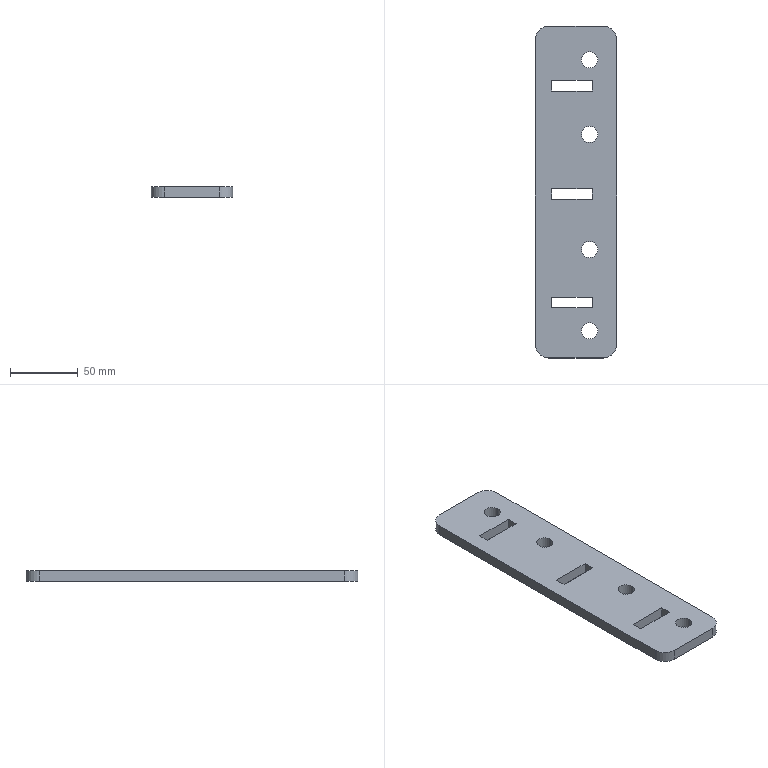Part | SolidWorks | features Fillet 1, FlatPattern 1, SMBaseFlange 1, SheetMetal 1 | 1 solid | 30 faces | box 60 x 245 x 8 mm | volume 107534 mm3 | plane 18 | cylinder 12 | commonest cylinder face diameters 12 x8 20 x4
STEP:
#1=CARTESIAN_POINT('',(88.081,95.,8.));
#2=VERTEX_POINT('',#1);
#3=CARTESIAN_POINT('',(100.081,95.,8.));
#4=VERTEX_POINT('',#3);
#5=CARTESIAN_POINT('',(94.081,95.,8.));
#6=DIRECTION('',(0.,0.,1.));
#7=DIRECTION('',(1.,0.,0.));
#8=AXIS2_PLACEMENT_3D('',#5,#6,#7);
#9=CIRCLE('',#8,6.);
#10=EDGE_CURVE('',#2,#4,#9,.T.);
#11=ORIENTED_EDGE('',*,*,#10,.T.);
#12=CARTESIAN_POINT('',(100.081,95.,0.));
#13=VERTEX_POINT('',#12);
#14=CARTESIAN_POINT('',(100.081,95.,8.));
#15=DIRECTION('',(0.,0.,-1.));
#16=VECTOR('',#15,1000.);
#17=LINE('',#14,#16);
#18=EDGE_CURVE('',#4,#13,#17,.T.);
#19=ORIENTED_EDGE('',*,*,#18,.T.);
#20=CARTESIAN_POINT('',(88.081,95.,0.));
#21=VERTEX_POINT('',#20);
#22=CARTESIAN_POINT('',(94.081,95.,0.));
#23=DIRECTION('',(0.,0.,1.));
#24=DIRECTION('',(1.,0.,0.));
#25=AXIS2_PLACEMENT_3D('',#22,#23,#24);
#26=CIRCLE('',#25,6.);
#27=EDGE_CURVE('',#21,#13,#26,.T.);
#28=ORIENTED_EDGE('',*,*,#27,.F.);
#29=CARTESIAN_POINT('',(88.081,95.,8.));
#30=DIRECTION('',(0.,0.,-1.));
#31=VECTOR('',#30,1000.);
#32=LINE('',#29,#31);
#33=EDGE_CURVE('',#2,#21,#32,.T.);
#34=ORIENTED_EDGE('',*,*,#33,.F.);
#35=EDGE_LOOP('',(#11,#19,#28,#34));
#36=FACE_OUTER_BOUND('',#35,.T.);
#37=CARTESIAN_POINT('',(94.081,95.,8.));
#38=DIRECTION('',(0.,0.,-1.));
#39=DIRECTION('',(-1.,0.,0.));
#40=AXIS2_PLACEMENT_3D('',#37,#38,#39);
#41=CYLINDRICAL_SURFACE('',#40,6.);
#42=ADVANCED_FACE('',(#36),#41,.F.);
#43=CARTESIAN_POINT('',(88.081,40.,8.));
#44=VERTEX_POINT('',#43);
#45=CARTESIAN_POINT('',(100.081,40.,8.));
#46=VERTEX_POINT('',#45);
#47=CARTESIAN_POINT('',(94.081,40.,8.));
#48=DIRECTION('',(0.,0.,1.));
#49=DIRECTION('',(1.,0.,0.));
#50=AXIS2_PLACEMENT_3D('',#47,#48,#49);
#51=CIRCLE('',#50,6.);
#52=EDGE_CURVE('',#44,#46,#51,.T.);
#53=ORIENTED_EDGE('',*,*,#52,.T.);
#54=CARTESIAN_POINT('',(100.081,40.,0.));
#55=VERTEX_POINT('',#54);
#56=CARTESIAN_POINT('',(100.081,40.,8.));
#57=DIRECTION('',(0.,0.,-1.));
#58=VECTOR('',#57,1000.);
#59=LINE('',#56,#58);
#60=EDGE_CURVE('',#46,#55,#59,.T.);
#61=ORIENTED_EDGE('',*,*,#60,.T.);
#62=CARTESIAN_POINT('',(88.081,40.,0.));
#63=VERTEX_POINT('',#62);
#64=CARTESIAN_POINT('',(94.081,40.,0.));
#65=DIRECTION('',(0.,0.,1.));
#66=DIRECTION('',(1.,0.,0.));
#67=AXIS2_PLACEMENT_3D('',#64,#65,#66);
#68=CIRCLE('',#67,6.);
#69=EDGE_CURVE('',#63,#55,#68,.T.);
#70=ORIENTED_EDGE('',*,*,#69,.F.);
#71=CARTESIAN_POINT('',(88.081,40.,8.));
#72=DIRECTION('',(0.,0.,-1.));
#73=VECTOR('',#72,1000.);
#74=LINE('',#71,#73);
#75=EDGE_CURVE('',#44,#63,#74,.T.);
#76=ORIENTED_EDGE('',*,*,#75,.F.);
#77=EDGE_LOOP('',(#53,#61,#70,#76));
#78=FACE_OUTER_BOUND('',#77,.T.);
#79=CARTESIAN_POINT('',(94.081,40.,8.));
#80=DIRECTION('',(0.,0.,-1.));
#81=DIRECTION('',(-1.,0.,0.));
#82=AXIS2_PLACEMENT_3D('',#79,#80,#81);
#83=CYLINDRICAL_SURFACE('',#82,6.);
#84=ADVANCED_FACE('',(#78),#83,.F.);
#85=CARTESIAN_POINT('',(88.081,-45.,8.));
#86=VERTEX_POINT('',#85);
#87=CARTESIAN_POINT('',(100.081,-45.,8.));
#88=VERTEX_POINT('',#87);
#89=CARTESIAN_POINT('',(94.081,-45.,8.));
#90=DIRECTION('',(0.,0.,1.));
#91=DIRECTION('',(1.,0.,0.));
#92=AXIS2_PLACEMENT_3D('',#89,#90,#91);
#93=CIRCLE('',#92,6.);
#94=EDGE_CURVE('',#86,#88,#93,.T.);
#95=ORIENTED_EDGE('',*,*,#94,.T.);
#96=CARTESIAN_POINT('',(100.081,-45.,0.));
#97=VERTEX_POINT('',#96);
#98=CARTESIAN_POINT('',(100.081,-45.,8.));
#99=DIRECTION('',(0.,0.,-1.));
#100=VECTOR('',#99,1000.);
#101=LINE('',#98,#100);
#102=EDGE_CURVE('',#88,#97,#101,.T.);
#103=ORIENTED_EDGE('',*,*,#102,.T.);
#104=CARTESIAN_POINT('',(88.081,-45.,0.));
#105=VERTEX_POINT('',#104);
#106=CARTESIAN_POINT('',(94.081,-45.,0.));
#107=DIRECTION('',(0.,0.,1.));
#108=DIRECTION('',(1.,0.,0.));
#109=AXIS2_PLACEMENT_3D('',#106,#107,#108);
#110=CIRCLE('',#109,6.);
#111=EDGE_CURVE('',#105,#97,#110,.T.);
#112=ORIENTED_EDGE('',*,*,#111,.F.);
#113=CARTESIAN_POINT('',(88.081,-45.,8.));
#114=DIRECTION('',(0.,0.,-1.));
#115=VECTOR('',#114,1000.);
#116=LINE('',#113,#115);
#117=EDGE_CURVE('',#86,#105,#116,.T.);
#118=ORIENTED_EDGE('',*,*,#117,.F.);
#119=EDGE_LOOP('',(#95,#103,#112,#118));
#120=FACE_OUTER_BOUND('',#119,.T.);
#121=CARTESIAN_POINT('',(94.081,-45.,8.));
#122=DIRECTION('',(0.,0.,-1.));
#123=DIRECTION('',(-1.,0.,0.));
#124=AXIS2_PLACEMENT_3D('',#121,#122,#123);
#125=CYLINDRICAL_SURFACE('',#124,6.);
#126=ADVANCED_FACE('',(#120),#125,.F.);
#127=CARTESIAN_POINT('',(88.081,-105.,8.));
#128=VERTEX_POINT('',#127);
#129=CARTESIAN_POINT('',(100.081,-105.,8.));
#130=VERTEX_POINT('',#129);
#131=CARTESIAN_POINT('',(94.081,-105.,8.));
#132=DIRECTION('',(0.,0.,1.));
#133=DIRECTION('',(1.,0.,0.));
#134=AXIS2_PLACEMENT_3D('',#131,#132,#133);
#135=CIRCLE('',#134,6.);
#136=EDGE_CURVE('',#128,#130,#135,.T.);
#137=ORIENTED_EDGE('',*,*,#136,.T.);
#138=CARTESIAN_POINT('',(100.081,-105.,0.));
#139=VERTEX_POINT('',#138);
#140=CARTESIAN_POINT('',(100.081,-105.,8.));
#141=DIRECTION('',(0.,0.,-1.));
#142=VECTOR('',#141,1000.);
#143=LINE('',#140,#142);
#144=EDGE_CURVE('',#130,#139,#143,.T.);
#145=ORIENTED_EDGE('',*,*,#144,.T.);
#146=CARTESIAN_POINT('',(88.081,-105.,0.));
#147=VERTEX_POINT('',#146);
#148=CARTESIAN_POINT('',(94.081,-105.,0.));
#149=DIRECTION('',(0.,0.,1.));
#150=DIRECTION('',(1.,0.,0.));
#151=AXIS2_PLACEMENT_3D('',#148,#149,#150);
#152=CIRCLE('',#151,6.);
#153=EDGE_CURVE('',#147,#139,#152,.T.);
#154=ORIENTED_EDGE('',*,*,#153,.F.);
#155=CARTESIAN_POINT('',(88.081,-105.,8.));
#156=DIRECTION('',(0.,0.,-1.));
#157=VECTOR('',#156,1000.);
#158=LINE('',#155,#157);
#159=EDGE_CURVE('',#128,#147,#158,.T.);
#160=ORIENTED_EDGE('',*,*,#159,.F.);
#161=EDGE_LOOP('',(#137,#145,#154,#160));
#162=FACE_OUTER_BOUND('',#161,.T.);
#163=CARTESIAN_POINT('',(94.081,-105.,8.));
#164=DIRECTION('',(0.,0.,-1.));
#165=DIRECTION('',(-1.,0.,0.));
#166=AXIS2_PLACEMENT_3D('',#163,#164,#165);
#167=CYLINDRICAL_SURFACE('',#166,6.);
#168=ADVANCED_FACE('',(#162),#167,.F.);
#169=ORIENTED_EDGE('',*,*,#52,.F.);
#170=CARTESIAN_POINT('',(94.081,40.,8.));
#171=DIRECTION('',(0.,0.,1.));
#172=DIRECTION('',(1.,0.,0.));
#173=AXIS2_PLACEMENT_3D('',#170,#171,#172);
#174=CIRCLE('',#173,6.);
#175=EDGE_CURVE('',#46,#44,#174,.T.);
#176=ORIENTED_EDGE('',*,*,#175,.F.);
#177=EDGE_LOOP('',(#169,#176));
#178=FACE_BOUND('',#177,.T.);
#179=ORIENTED_EDGE('',*,*,#136,.F.);
#180=CARTESIAN_POINT('',(94.081,-105.,8.));
#181=DIRECTION('',(0.,0.,1.));
#182=DIRECTION('',(1.,0.,0.));
#183=AXIS2_PLACEMENT_3D('',#180,#181,#182);
#184=CIRCLE('',#183,6.);
#185=EDGE_CURVE('',#130,#128,#184,.T.);
#186=ORIENTED_EDGE('',*,*,#185,.F.);
#187=EDGE_LOOP('',(#179,#186));
#188=FACE_BOUND('',#187,.T.);
#189=CARTESIAN_POINT('',(114.081,-115.,8.));
#190=VERTEX_POINT('',#189);
#191=CARTESIAN_POINT('',(114.081,110.,8.));
#192=VERTEX_POINT('',#191);
#193=CARTESIAN_POINT('',(114.081,-125.,8.));
#194=DIRECTION('',(0.,1.,0.));
#195=VECTOR('',#194,1000.);
#196=LINE('',#193,#195);
#197=EDGE_CURVE('',#190,#192,#196,.T.);
#198=ORIENTED_EDGE('',*,*,#197,.T.);
#199=CARTESIAN_POINT('',(104.081,120.,8.));
#200=VERTEX_POINT('',#199);
#201=CARTESIAN_POINT('',(104.081,110.,8.));
#202=DIRECTION('',(0.,0.,1.));
#203=DIRECTION('',(1.,0.,0.));
#204=AXIS2_PLACEMENT_3D('',#201,#202,#203);
#205=CIRCLE('',#204,10.);
#206=EDGE_CURVE('',#192,#200,#205,.T.);
#207=ORIENTED_EDGE('',*,*,#206,.T.);
#208=CARTESIAN_POINT('',(64.081,120.,8.));
#209=VERTEX_POINT('',#208);
#210=CARTESIAN_POINT('',(114.081,120.,8.));
#211=DIRECTION('',(-1.,0.,0.));
#212=VECTOR('',#211,1000.);
#213=LINE('',#210,#212);
#214=EDGE_CURVE('',#200,#209,#213,.T.);
#215=ORIENTED_EDGE('',*,*,#214,.T.);
#216=CARTESIAN_POINT('',(54.081,110.,8.));
#217=VERTEX_POINT('',#216);
#218=CARTESIAN_POINT('',(64.081,110.,8.));
#219=DIRECTION('',(0.,0.,1.));
#220=DIRECTION('',(1.,0.,0.));
#221=AXIS2_PLACEMENT_3D('',#218,#219,#220);
#222=CIRCLE('',#221,10.);
#223=EDGE_CURVE('',#209,#217,#222,.T.);
#224=ORIENTED_EDGE('',*,*,#223,.T.);
#225=CARTESIAN_POINT('',(54.081,-115.,8.));
#226=VERTEX_POINT('',#225);
#227=CARTESIAN_POINT('',(54.081,120.,8.));
#228=DIRECTION('',(0.,-1.,0.));
#229=VECTOR('',#228,1000.);
#230=LINE('',#227,#229);
#231=EDGE_CURVE('',#217,#226,#230,.T.);
#232=ORIENTED_EDGE('',*,*,#231,.T.);
#233=CARTESIAN_POINT('',(64.081,-125.,8.));
#234=VERTEX_POINT('',#233);
#235=CARTESIAN_POINT('',(64.081,-115.,8.));
#236=DIRECTION('',(0.,0.,1.));
#237=DIRECTION('',(1.,0.,0.));
#238=AXIS2_PLACEMENT_3D('',#235,#236,#237);
#239=CIRCLE('',#238,10.);
#240=EDGE_CURVE('',#226,#234,#239,.T.);
#241=ORIENTED_EDGE('',*,*,#240,.T.);
#242=CARTESIAN_POINT('',(104.081,-125.,8.));
#243=VERTEX_POINT('',#242);
#244=CARTESIAN_POINT('',(54.081,-125.,8.));
#245=DIRECTION('',(1.,0.,0.));
#246=VECTOR('',#245,1000.);
#247=LINE('',#244,#246);
#248=EDGE_CURVE('',#234,#243,#247,.T.);
#249=ORIENTED_EDGE('',*,*,#248,.T.);
#250=CARTESIAN_POINT('',(104.081,-115.,8.));
#251=DIRECTION('',(0.,0.,1.));
#252=DIRECTION('',(1.,0.,0.));
#253=AXIS2_PLACEMENT_3D('',#250,#251,#252);
#254=CIRCLE('',#253,10.);
#255=EDGE_CURVE('',#243,#190,#254,.T.);
#256=ORIENTED_EDGE('',*,*,#255,.T.);
#257=EDGE_LOOP('',(#198,#207,#215,#224,#232,#241,#249,#256));
#258=FACE_OUTER_BOUND('',#257,.T.);
#259=CARTESIAN_POINT('',(96.081,-88.,8.));
#260=VERTEX_POINT('',#259);
#261=CARTESIAN_POINT('',(96.081,-80.,8.));
#262=VERTEX_POINT('',#261);
#263=CARTESIAN_POINT('',(96.081,-80.,8.));
#264=DIRECTION('',(0.,1.,0.));
#265=VECTOR('',#264,1000.);
#266=LINE('',#263,#265);
#267=EDGE_CURVE('',#260,#262,#266,.T.);
#268=ORIENTED_EDGE('',*,*,#267,.F.);
#269=CARTESIAN_POINT('',(66.081,-88.,8.));
#270=VERTEX_POINT('',#269);
#271=CARTESIAN_POINT('',(96.081,-88.,8.));
#272=DIRECTION('',(1.,0.,0.));
#273=VECTOR('',#272,1000.);
#274=LINE('',#271,#273);
#275=EDGE_CURVE('',#270,#260,#274,.T.);
#276=ORIENTED_EDGE('',*,*,#275,.F.);
#277=CARTESIAN_POINT('',(66.081,-80.,8.));
#278=VERTEX_POINT('',#277);
#279=CARTESIAN_POINT('',(66.081,-88.,8.));
#280=DIRECTION('',(0.,-1.,0.));
#281=VECTOR('',#280,1000.);
#282=LINE('',#279,#281);
#283=EDGE_CURVE('',#278,#270,#282,.T.);
#284=ORIENTED_EDGE('',*,*,#283,.F.);
#285=CARTESIAN_POINT('',(66.081,-80.,8.));
#286=DIRECTION('',(-1.,0.,0.));
#287=VECTOR('',#286,1000.);
#288=LINE('',#285,#287);
#289=EDGE_CURVE('',#262,#278,#288,.T.);
#290=ORIENTED_EDGE('',*,*,#289,.F.);
#291=EDGE_LOOP('',(#268,#276,#284,#290));
#292=FACE_BOUND('',#291,.T.);
#293=CARTESIAN_POINT('',(96.081,-8.,8.));
#294=VERTEX_POINT('',#293);
#295=CARTESIAN_POINT('',(96.081,0.,8.));
#296=VERTEX_POINT('',#295);
#297=CARTESIAN_POINT('',(96.081,0.,8.));
#298=DIRECTION('',(0.,1.,0.));
#299=VECTOR('',#298,1000.);
#300=LINE('',#297,#299);
#301=EDGE_CURVE('',#294,#296,#300,.T.);
#302=ORIENTED_EDGE('',*,*,#301,.F.);
#303=CARTESIAN_POINT('',(66.081,-8.,8.));
#304=VERTEX_POINT('',#303);
#305=CARTESIAN_POINT('',(96.081,-8.,8.));
#306=DIRECTION('',(1.,0.,0.));
#307=VECTOR('',#306,1000.);
#308=LINE('',#305,#307);
#309=EDGE_CURVE('',#304,#294,#308,.T.);
#310=ORIENTED_EDGE('',*,*,#309,.F.);
#311=CARTESIAN_POINT('',(66.081,0.,8.));
#312=VERTEX_POINT('',#311);
#313=CARTESIAN_POINT('',(66.081,-8.,8.));
#314=DIRECTION('',(0.,-1.,0.));
#315=VECTOR('',#314,1000.);
#316=LINE('',#313,#315);
#317=EDGE_CURVE('',#312,#304,#316,.T.);
#318=ORIENTED_EDGE('',*,*,#317,.F.);
#319=CARTESIAN_POINT('',(66.081,0.,8.));
#320=DIRECTION('',(-1.,0.,0.));
#321=VECTOR('',#320,1000.);
#322=LINE('',#319,#321);
#323=EDGE_CURVE('',#296,#312,#322,.T.);
#324=ORIENTED_EDGE('',*,*,#323,.F.);
#325=EDGE_LOOP('',(#302,#310,#318,#324));
#326=FACE_BOUND('',#325,.T.);
#327=CARTESIAN_POINT('',(96.081,72.,8.));
#328=VERTEX_POINT('',#327);
#329=CARTESIAN_POINT('',(96.081,80.,8.));
#330=VERTEX_POINT('',#329);
#331=CARTESIAN_POINT('',(96.081,80.,8.));
#332=DIRECTION('',(0.,1.,0.));
#333=VECTOR('',#332,1000.);
#334=LINE('',#331,#333);
#335=EDGE_CURVE('',#328,#330,#334,.T.);
#336=ORIENTED_EDGE('',*,*,#335,.F.);
#337=CARTESIAN_POINT('',(66.081,72.,8.));
#338=VERTEX_POINT('',#337);
#339=CARTESIAN_POINT('',(96.081,72.,8.));
#340=DIRECTION('',(1.,0.,0.));
#341=VECTOR('',#340,1000.);
#342=LINE('',#339,#341);
#343=EDGE_CURVE('',#338,#328,#342,.T.);
#344=ORIENTED_EDGE('',*,*,#343,.F.);
#345=CARTESIAN_POINT('',(66.081,80.,8.));
#346=VERTEX_POINT('',#345);
#347=CARTESIAN_POINT('',(66.081,72.,8.));
#348=DIRECTION('',(0.,-1.,0.));
#349=VECTOR('',#348,1000.);
#350=LINE('',#347,#349);
#351=EDGE_CURVE('',#346,#338,#350,.T.);
#352=ORIENTED_EDGE('',*,*,#351,.F.);
#353=CARTESIAN_POINT('',(66.081,80.,8.));
#354=DIRECTION('',(-1.,0.,0.));
#355=VECTOR('',#354,1000.);
#356=LINE('',#353,#355);
#357=EDGE_CURVE('',#330,#346,#356,.T.);
#358=ORIENTED_EDGE('',*,*,#357,.F.);
#359=EDGE_LOOP('',(#336,#344,#352,#358));
#360=FACE_BOUND('',#359,.T.);
#361=ORIENTED_EDGE('',*,*,#94,.F.);
#362=CARTESIAN_POINT('',(94.081,-45.,8.));
#363=DIRECTION('',(0.,0.,1.));
#364=DIRECTION('',(1.,0.,0.));
#365=AXIS2_PLACEMENT_3D('',#362,#363,#364);
#366=CIRCLE('',#365,6.);
#367=EDGE_CURVE('',#88,#86,#366,.T.);
#368=ORIENTED_EDGE('',*,*,#367,.F.);
#369=EDGE_LOOP('',(#361,#368));
#370=FACE_BOUND('',#369,.T.);
#371=ORIENTED_EDGE('',*,*,#10,.F.);
#372=CARTESIAN_POINT('',(94.081,95.,8.));
#373=DIRECTION('',(0.,0.,1.));
#374=DIRECTION('',(1.,0.,0.));
#375=AXIS2_PLACEMENT_3D('',#372,#373,#374);
#376=CIRCLE('',#375,6.);
#377=EDGE_CURVE('',#4,#2,#376,.T.);
#378=ORIENTED_EDGE('',*,*,#377,.F.);
#379=EDGE_LOOP('',(#371,#378));
#380=FACE_BOUND('',#379,.T.);
#381=CARTESIAN_POINT('',(0.,0.,8.));
#382=DIRECTION('',(0.,0.,1.));
#383=DIRECTION('',(1.,0.,0.));
#384=AXIS2_PLACEMENT_3D('',#381,#382,#383);
#385=PLANE('',#384);
#386=ADVANCED_FACE('',(#178,#188,#258,#292,#326,#360,#370,#380),#385,.T.);
#387=CARTESIAN_POINT('',(66.081,-8.,0.));
#388=VERTEX_POINT('',#387);
#389=CARTESIAN_POINT('',(96.081,-8.,0.));
#390=VERTEX_POINT('',#389);
#391=CARTESIAN_POINT('',(96.081,-8.,0.));
#392=DIRECTION('',(1.,0.,0.));
#393=VECTOR('',#392,1000.);
#394=LINE('',#391,#393);
#395=EDGE_CURVE('',#388,#390,#394,.T.);
#396=ORIENTED_EDGE('',*,*,#395,.T.);
#397=CARTESIAN_POINT('',(96.081,0.,0.));
#398=VERTEX_POINT('',#397);
#399=CARTESIAN_POINT('',(96.081,0.,0.));
#400=DIRECTION('',(0.,1.,0.));
#401=VECTOR('',#400,1000.);
#402=LINE('',#399,#401);
#403=EDGE_CURVE('',#390,#398,#402,.T.);
#404=ORIENTED_EDGE('',*,*,#403,.T.);
#405=CARTESIAN_POINT('',(66.081,0.,0.));
#406=VERTEX_POINT('',#405);
#407=CARTESIAN_POINT('',(66.081,0.,0.));
#408=DIRECTION('',(-1.,0.,0.));
#409=VECTOR('',#408,1000.);
#410=LINE('',#407,#409);
#411=EDGE_CURVE('',#398,#406,#410,.T.);
#412=ORIENTED_EDGE('',*,*,#411,.T.);
#413=CARTESIAN_POINT('',(66.081,-8.,0.));
#414=DIRECTION('',(0.,-1.,0.));
#415=VECTOR('',#414,1000.);
#416=LINE('',#413,#415);
#417=EDGE_CURVE('',#406,#388,#416,.T.);
#418=ORIENTED_EDGE('',*,*,#417,.T.);
#419=EDGE_LOOP('',(#396,#404,#412,#418));
#420=FACE_BOUND('',#419,.T.);
#421=CARTESIAN_POINT('',(104.081,120.,0.));
#422=VERTEX_POINT('',#421);
#423=CARTESIAN_POINT('',(64.081,120.,0.));
#424=VERTEX_POINT('',#423);
#425=CARTESIAN_POINT('',(114.081,120.,0.));
#426=DIRECTION('',(-1.,0.,0.));
#427=VECTOR('',#426,1000.);
#428=LINE('',#425,#427);
#429=EDGE_CURVE('',#422,#424,#428,.T.);
#430=ORIENTED_EDGE('',*,*,#429,.F.);
#431=CARTESIAN_POINT('',(114.081,110.,0.));
#432=VERTEX_POINT('',#431);
#433=CARTESIAN_POINT('',(104.081,110.,0.));
#434=DIRECTION('',(0.,0.,-1.));
#435=DIRECTION('',(1.,0.,0.));
#436=AXIS2_PLACEMENT_3D('',#433,#434,#435);
#437=CIRCLE('',#436,10.);
#438=EDGE_CURVE('',#422,#432,#437,.T.);
#439=ORIENTED_EDGE('',*,*,#438,.T.);
#440=CARTESIAN_POINT('',(114.081,-115.,0.));
#441=VERTEX_POINT('',#440);
#442=CARTESIAN_POINT('',(114.081,-125.,0.));
#443=DIRECTION('',(0.,1.,0.));
#444=VECTOR('',#443,1000.);
#445=LINE('',#442,#444);
#446=EDGE_CURVE('',#441,#432,#445,.T.);
#447=ORIENTED_EDGE('',*,*,#446,.F.);
#448=CARTESIAN_POINT('',(104.081,-125.,0.));
#449=VERTEX_POINT('',#448);
#450=CARTESIAN_POINT('',(104.081,-115.,0.));
#451=DIRECTION('',(0.,0.,-1.));
#452=DIRECTION('',(1.,0.,0.));
#453=AXIS2_PLACEMENT_3D('',#450,#451,#452);
#454=CIRCLE('',#453,10.);
#455=EDGE_CURVE('',#441,#449,#454,.T.);
#456=ORIENTED_EDGE('',*,*,#455,.T.);
#457=CARTESIAN_POINT('',(64.081,-125.,0.));
#458=VERTEX_POINT('',#457);
#459=CARTESIAN_POINT('',(54.081,-125.,0.));
#460=DIRECTION('',(1.,0.,0.));
#461=VECTOR('',#460,1000.);
#462=LINE('',#459,#461);
#463=EDGE_CURVE('',#458,#449,#462,.T.);
#464=ORIENTED_EDGE('',*,*,#463,.F.);
#465=CARTESIAN_POINT('',(54.081,-115.,0.));
#466=VERTEX_POINT('',#465);
#467=CARTESIAN_POINT('',(64.081,-115.,0.));
#468=DIRECTION('',(0.,0.,-1.));
#469=DIRECTION('',(1.,0.,0.));
#470=AXIS2_PLACEMENT_3D('',#467,#468,#469);
#471=CIRCLE('',#470,10.);
#472=EDGE_CURVE('',#458,#466,#471,.T.);
#473=ORIENTED_EDGE('',*,*,#472,.T.);
#474=CARTESIAN_POINT('',(54.081,110.,0.));
#475=VERTEX_POINT('',#474);
#476=CARTESIAN_POINT('',(54.081,120.,0.));
#477=DIRECTION('',(0.,-1.,0.));
#478=VECTOR('',#477,1000.);
#479=LINE('',#476,#478);
#480=EDGE_CURVE('',#475,#466,#479,.T.);
#481=ORIENTED_EDGE('',*,*,#480,.F.);
#482=CARTESIAN_POINT('',(64.081,110.,0.));
#483=DIRECTION('',(0.,0.,-1.));
#484=DIRECTION('',(1.,0.,0.));
#485=AXIS2_PLACEMENT_3D('',#482,#483,#484);
#486=CIRCLE('',#485,10.);
#487=EDGE_CURVE('',#475,#424,#486,.T.);
#488=ORIENTED_EDGE('',*,*,#487,.T.);
#489=EDGE_LOOP('',(#430,#439,#447,#456,#464,#473,#481,#488));
#490=FACE_OUTER_BOUND('',#489,.T.);
#491=CARTESIAN_POINT('',(66.081,-88.,0.));
#492=VERTEX_POINT('',#491);
#493=CARTESIAN_POINT('',(96.081,-88.,0.));
#494=VERTEX_POINT('',#493);
#495=CARTESIAN_POINT('',(96.081,-88.,0.));
#496=DIRECTION('',(1.,0.,0.));
#497=VECTOR('',#496,1000.);
#498=LINE('',#495,#497);
#499=EDGE_CURVE('',#492,#494,#498,.T.);
#500=ORIENTED_EDGE('',*,*,#499,.T.);
#501=CARTESIAN_POINT('',(96.081,-80.,0.));
#502=VERTEX_POINT('',#501);
#503=CARTESIAN_POINT('',(96.081,-80.,0.));
#504=DIRECTION('',(0.,1.,0.));
#505=VECTOR('',#504,1000.);
#506=LINE('',#503,#505);
#507=EDGE_CURVE('',#494,#502,#506,.T.);
#508=ORIENTED_EDGE('',*,*,#507,.T.);
#509=CARTESIAN_POINT('',(66.081,-80.,0.));
#510=VERTEX_POINT('',#509);
#511=CARTESIAN_POINT('',(66.081,-80.,0.));
#512=DIRECTION('',(-1.,0.,0.));
#513=VECTOR('',#512,1000.);
#514=LINE('',#511,#513);
#515=EDGE_CURVE('',#502,#510,#514,.T.);
#516=ORIENTED_EDGE('',*,*,#515,.T.);
#517=CARTESIAN_POINT('',(66.081,-88.,0.));
#518=DIRECTION('',(0.,-1.,0.));
#519=VECTOR('',#518,1000.);
#520=LINE('',#517,#519);
#521=EDGE_CURVE('',#510,#492,#520,.T.);
#522=ORIENTED_EDGE('',*,*,#521,.T.);
#523=EDGE_LOOP('',(#500,#508,#516,#522));
#524=FACE_BOUND('',#523,.T.);
#525=CARTESIAN_POINT('',(66.081,72.,0.));
#526=VERTEX_POINT('',#525);
#527=CARTESIAN_POINT('',(96.081,72.,0.));
#528=VERTEX_POINT('',#527);
#529=CARTESIAN_POINT('',(96.081,72.,0.));
#530=DIRECTION('',(1.,0.,0.));
#531=VECTOR('',#530,1000.);
#532=LINE('',#529,#531);
#533=EDGE_CURVE('',#526,#528,#532,.T.);
#534=ORIENTED_EDGE('',*,*,#533,.T.);
#535=CARTESIAN_POINT('',(96.081,80.,0.));
#536=VERTEX_POINT('',#535);
#537=CARTESIAN_POINT('',(96.081,80.,0.));
#538=DIRECTION('',(0.,1.,0.));
#539=VECTOR('',#538,1000.);
#540=LINE('',#537,#539);
#541=EDGE_CURVE('',#528,#536,#540,.T.);
#542=ORIENTED_EDGE('',*,*,#541,.T.);
#543=CARTESIAN_POINT('',(66.081,80.,0.));
#544=VERTEX_POINT('',#543);
#545=CARTESIAN_POINT('',(66.081,80.,0.));
#546=DIRECTION('',(-1.,0.,0.));
#547=VECTOR('',#546,1000.);
#548=LINE('',#545,#547);
#549=EDGE_CURVE('',#536,#544,#548,.T.);
#550=ORIENTED_EDGE('',*,*,#549,.T.);
#551=CARTESIAN_POINT('',(66.081,72.,0.));
#552=DIRECTION('',(0.,-1.,0.));
#553=VECTOR('',#552,1000.);
#554=LINE('',#551,#553);
#555=EDGE_CURVE('',#544,#526,#554,.T.);
#556=ORIENTED_EDGE('',*,*,#555,.T.);
#557=EDGE_LOOP('',(#534,#542,#550,#556));
#558=FACE_BOUND('',#557,.T.);
#559=ORIENTED_EDGE('',*,*,#153,.T.);
#560=CARTESIAN_POINT('',(94.081,-105.,0.));
#561=DIRECTION('',(0.,0.,1.));
#562=DIRECTION('',(1.,0.,0.));
#563=AXIS2_PLACEMENT_3D('',#560,#561,#562);
#564=CIRCLE('',#563,6.);
#565=EDGE_CURVE('',#139,#147,#564,.T.);
#566=ORIENTED_EDGE('',*,*,#565,.T.);
#567=EDGE_LOOP('',(#559,#566));
#568=FACE_BOUND('',#567,.T.);
#569=ORIENTED_EDGE('',*,*,#111,.T.);
#570=CARTESIAN_POINT('',(94.081,-45.,0.));
#571=DIRECTION('',(0.,0.,1.));
#572=DIRECTION('',(1.,0.,0.));
#573=AXIS2_PLACEMENT_3D('',#570,#571,#572);
#574=CIRCLE('',#573,6.);
#575=EDGE_CURVE('',#97,#105,#574,.T.);
#576=ORIENTED_EDGE('',*,*,#575,.T.);
#577=EDGE_LOOP('',(#569,#576));
#578=FACE_BOUND('',#577,.T.);
#579=ORIENTED_EDGE('',*,*,#69,.T.);
#580=CARTESIAN_POINT('',(94.081,40.,0.));
#581=DIRECTION('',(0.,0.,1.));
#582=DIRECTION('',(1.,0.,0.));
#583=AXIS2_PLACEMENT_3D('',#580,#581,#582);
#584=CIRCLE('',#583,6.);
#585=EDGE_CURVE('',#55,#63,#584,.T.);
#586=ORIENTED_EDGE('',*,*,#585,.T.);
#587=EDGE_LOOP('',(#579,#586));
#588=FACE_BOUND('',#587,.T.);
#589=ORIENTED_EDGE('',*,*,#27,.T.);
#590=CARTESIAN_POINT('',(94.081,95.,0.));
#591=DIRECTION('',(0.,0.,1.));
#592=DIRECTION('',(1.,0.,0.));
#593=AXIS2_PLACEMENT_3D('',#590,#591,#592);
#594=CIRCLE('',#593,6.);
#595=EDGE_CURVE('',#13,#21,#594,.T.);
#596=ORIENTED_EDGE('',*,*,#595,.T.);
#597=EDGE_LOOP('',(#589,#596));
#598=FACE_BOUND('',#597,.T.);
#599=CARTESIAN_POINT('',(0.,0.,0.));
#600=DIRECTION('',(0.,0.,1.));
#601=DIRECTION('',(1.,0.,0.));
#602=AXIS2_PLACEMENT_3D('',#599,#600,#601);
#603=PLANE('',#602);
#604=ADVANCED_FACE('',(#420,#490,#524,#558,#568,#578,#588,#598),#603,.F.);
#605=ORIENTED_EDGE('',*,*,#463,.T.);
#606=CARTESIAN_POINT('',(104.081,-125.,8.));
#607=DIRECTION('',(0.,0.,1.));
#608=VECTOR('',#607,1000.);
#609=LINE('',#606,#608);
#610=EDGE_CURVE('',#449,#243,#609,.T.);
#611=ORIENTED_EDGE('',*,*,#610,.T.);
#612=ORIENTED_EDGE('',*,*,#248,.F.);
#613=CARTESIAN_POINT('',(64.081,-125.,8.));
#614=DIRECTION('',(0.,0.,-1.));
#615=VECTOR('',#614,1000.);
#616=LINE('',#613,#615);
#617=EDGE_CURVE('',#234,#458,#616,.T.);
#618=ORIENTED_EDGE('',*,*,#617,.T.);
#619=EDGE_LOOP('',(#605,#611,#612,#618));
#620=FACE_OUTER_BOUND('',#619,.T.);
#621=CARTESIAN_POINT('',(54.081,-125.,8.));
#622=DIRECTION('',(0.,1.,0.));
#623=DIRECTION('',(0.,0.,1.));
#624=AXIS2_PLACEMENT_3D('',#621,#622,#623);
#625=PLANE('',#624);
#626=ADVANCED_FACE('',(#620),#625,.F.);
#627=ORIENTED_EDGE('',*,*,#446,.T.);
#628=CARTESIAN_POINT('',(114.081,110.,8.));
#629=DIRECTION('',(0.,0.,1.));
#630=VECTOR('',#629,1000.);
#631=LINE('',#628,#630);
#632=EDGE_CURVE('',#432,#192,#631,.T.);
#633=ORIENTED_EDGE('',*,*,#632,.T.);
#634=ORIENTED_EDGE('',*,*,#197,.F.);
#635=CARTESIAN_POINT('',(114.081,-115.,8.));
#636=DIRECTION('',(0.,0.,-1.));
#637=VECTOR('',#636,1000.);
#638=LINE('',#635,#637);
#639=EDGE_CURVE('',#190,#441,#638,.T.);
#640=ORIENTED_EDGE('',*,*,#639,.T.);
#641=EDGE_LOOP('',(#627,#633,#634,#640));
#642=FACE_OUTER_BOUND('',#641,.T.);
#643=CARTESIAN_POINT('',(114.081,-125.,8.));
#644=DIRECTION('',(-1.,0.,0.));
#645=DIRECTION('',(0.,0.,1.));
#646=AXIS2_PLACEMENT_3D('',#643,#644,#645);
#647=PLANE('',#646);
#648=ADVANCED_FACE('',(#642),#647,.F.);
#649=ORIENTED_EDGE('',*,*,#214,.F.);
#650=CARTESIAN_POINT('',(104.081,120.,8.));
#651=DIRECTION('',(0.,0.,-1.));
#652=VECTOR('',#651,1000.);
#653=LINE('',#650,#652);
#654=EDGE_CURVE('',#200,#422,#653,.T.);
#655=ORIENTED_EDGE('',*,*,#654,.T.);
#656=ORIENTED_EDGE('',*,*,#429,.T.);
#657=CARTESIAN_POINT('',(64.081,120.,8.));
#658=DIRECTION('',(0.,0.,1.));
#659=VECTOR('',#658,1000.);
#660=LINE('',#657,#659);
#661=EDGE_CURVE('',#424,#209,#660,.T.);
#662=ORIENTED_EDGE('',*,*,#661,.T.);
#663=EDGE_LOOP('',(#649,#655,#656,#662));
#664=FACE_OUTER_BOUND('',#663,.T.);
#665=CARTESIAN_POINT('',(114.081,120.,8.));
#666=DIRECTION('',(0.,-1.,0.));
#667=DIRECTION('',(1.,0.,0.));
#668=AXIS2_PLACEMENT_3D('',#665,#666,#667);
#669=PLANE('',#668);
#670=ADVANCED_FACE('',(#664),#669,.F.);
#671=ORIENTED_EDGE('',*,*,#480,.T.);
#672=CARTESIAN_POINT('',(54.081,-115.,8.));
#673=DIRECTION('',(0.,0.,1.));
#674=VECTOR('',#673,1000.);
#675=LINE('',#672,#674);
#676=EDGE_CURVE('',#466,#226,#675,.T.);
#677=ORIENTED_EDGE('',*,*,#676,.T.);
#678=ORIENTED_EDGE('',*,*,#231,.F.);
#679=CARTESIAN_POINT('',(54.081,110.,8.));
#680=DIRECTION('',(0.,0.,-1.));
#681=VECTOR('',#680,1000.);
#682=LINE('',#679,#681);
#683=EDGE_CURVE('',#217,#475,#682,.T.);
#684=ORIENTED_EDGE('',*,*,#683,.T.);
#685=EDGE_LOOP('',(#671,#677,#678,#684));
#686=FACE_OUTER_BOUND('',#685,.T.);
#687=CARTESIAN_POINT('',(54.081,120.,8.));
#688=DIRECTION('',(1.,0.,0.));
#689=DIRECTION('',(0.,1.,0.));
#690=AXIS2_PLACEMENT_3D('',#687,#688,#689);
#691=PLANE('',#690);
#692=ADVANCED_FACE('',(#686),#691,.F.);
#693=ORIENTED_EDGE('',*,*,#499,.F.);
#694=CARTESIAN_POINT('',(66.081,-88.,8.));
#695=DIRECTION('',(0.,0.,-1.));
#696=VECTOR('',#695,1000.);
#697=LINE('',#694,#696);
#698=EDGE_CURVE('',#270,#492,#697,.T.);
#699=ORIENTED_EDGE('',*,*,#698,.F.);
#700=ORIENTED_EDGE('',*,*,#275,.T.);
#701=CARTESIAN_POINT('',(96.081,-88.,8.));
#702=DIRECTION('',(0.,0.,-1.));
#703=VECTOR('',#702,1000.);
#704=LINE('',#701,#703);
#705=EDGE_CURVE('',#260,#494,#704,.T.);
#706=ORIENTED_EDGE('',*,*,#705,.T.);
#707=EDGE_LOOP('',(#693,#699,#700,#706));
#708=FACE_OUTER_BOUND('',#707,.T.);
#709=CARTESIAN_POINT('',(96.081,-88.,8.));
#710=DIRECTION('',(0.,1.,0.));
#711=DIRECTION('',(0.,0.,1.));
#712=AXIS2_PLACEMENT_3D('',#709,#710,#711);
#713=PLANE('',#712);
#714=ADVANCED_FACE('',(#708),#713,.T.);
#715=ORIENTED_EDGE('',*,*,#507,.F.);
#716=ORIENTED_EDGE('',*,*,#705,.F.);
#717=ORIENTED_EDGE('',*,*,#267,.T.);
#718=CARTESIAN_POINT('',(96.081,-80.,8.));
#719=DIRECTION('',(0.,0.,-1.));
#720=VECTOR('',#719,1000.);
#721=LINE('',#718,#720);
#722=EDGE_CURVE('',#262,#502,#721,.T.);
#723=ORIENTED_EDGE('',*,*,#722,.T.);
#724=EDGE_LOOP('',(#715,#716,#717,#723));
#725=FACE_OUTER_BOUND('',#724,.T.);
#726=CARTESIAN_POINT('',(96.081,-80.,8.));
#727=DIRECTION('',(-1.,0.,0.));
#728=DIRECTION('',(0.,0.,1.));
#729=AXIS2_PLACEMENT_3D('',#726,#727,#728);
#730=PLANE('',#729);
#731=ADVANCED_FACE('',(#725),#730,.T.);
#732=ORIENTED_EDGE('',*,*,#515,.F.);
#733=ORIENTED_EDGE('',*,*,#722,.F.);
#734=ORIENTED_EDGE('',*,*,#289,.T.);
#735=CARTESIAN_POINT('',(66.081,-80.,8.));
#736=DIRECTION('',(0.,0.,-1.));
#737=VECTOR('',#736,1000.);
#738=LINE('',#735,#737);
#739=EDGE_CURVE('',#278,#510,#738,.T.);
#740=ORIENTED_EDGE('',*,*,#739,.T.);
#741=EDGE_LOOP('',(#732,#733,#734,#740));
#742=FACE_OUTER_BOUND('',#741,.T.);
#743=CARTESIAN_POINT('',(66.081,-80.,8.));
#744=DIRECTION('',(0.,-1.,0.));
#745=DIRECTION('',(0.,0.,-1.));
#746=AXIS2_PLACEMENT_3D('',#743,#744,#745);
#747=PLANE('',#746);
#748=ADVANCED_FACE('',(#742),#747,.T.);
#749=ORIENTED_EDGE('',*,*,#521,.F.);
#750=ORIENTED_EDGE('',*,*,#739,.F.);
#751=ORIENTED_EDGE('',*,*,#283,.T.);
#752=ORIENTED_EDGE('',*,*,#698,.T.);
#753=EDGE_LOOP('',(#749,#750,#751,#752));
#754=FACE_OUTER_BOUND('',#753,.T.);
#755=CARTESIAN_POINT('',(66.081,-88.,8.));
#756=DIRECTION('',(1.,0.,0.));
#757=DIRECTION('',(0.,0.,-1.));
#758=AXIS2_PLACEMENT_3D('',#755,#756,#757);
#759=PLANE('',#758);
#760=ADVANCED_FACE('',(#754),#759,.T.);
#761=ORIENTED_EDGE('',*,*,#395,.F.);
#762=CARTESIAN_POINT('',(66.081,-8.,8.));
#763=DIRECTION('',(0.,0.,-1.));
#764=VECTOR('',#763,1000.);
#765=LINE('',#762,#764);
#766=EDGE_CURVE('',#304,#388,#765,.T.);
#767=ORIENTED_EDGE('',*,*,#766,.F.);
#768=ORIENTED_EDGE('',*,*,#309,.T.);
#769=CARTESIAN_POINT('',(96.081,-8.,8.));
#770=DIRECTION('',(0.,0.,-1.));
#771=VECTOR('',#770,1000.);
#772=LINE('',#769,#771);
#773=EDGE_CURVE('',#294,#390,#772,.T.);
#774=ORIENTED_EDGE('',*,*,#773,.T.);
#775=EDGE_LOOP('',(#761,#767,#768,#774));
#776=FACE_OUTER_BOUND('',#775,.T.);
#777=CARTESIAN_POINT('',(96.081,-8.,8.));
#778=DIRECTION('',(0.,1.,0.));
#779=DIRECTION('',(0.,0.,1.));
#780=AXIS2_PLACEMENT_3D('',#777,#778,#779);
#781=PLANE('',#780);
#782=ADVANCED_FACE('',(#776),#781,.T.);
#783=ORIENTED_EDGE('',*,*,#403,.F.);
#784=ORIENTED_EDGE('',*,*,#773,.F.);
#785=ORIENTED_EDGE('',*,*,#301,.T.);
#786=CARTESIAN_POINT('',(96.081,0.,8.));
#787=DIRECTION('',(0.,0.,-1.));
#788=VECTOR('',#787,1000.);
#789=LINE('',#786,#788);
#790=EDGE_CURVE('',#296,#398,#789,.T.);
#791=ORIENTED_EDGE('',*,*,#790,.T.);
#792=EDGE_LOOP('',(#783,#784,#785,#791));
#793=FACE_OUTER_BOUND('',#792,.T.);
#794=CARTESIAN_POINT('',(96.081,0.,8.));
#795=DIRECTION('',(-1.,0.,0.));
#796=DIRECTION('',(0.,0.,1.));
#797=AXIS2_PLACEMENT_3D('',#794,#795,#796);
#798=PLANE('',#797);
#799=ADVANCED_FACE('',(#793),#798,.T.);
#800=ORIENTED_EDGE('',*,*,#411,.F.);
#801=ORIENTED_EDGE('',*,*,#790,.F.);
#802=ORIENTED_EDGE('',*,*,#323,.T.);
#803=CARTESIAN_POINT('',(66.081,0.,8.));
#804=DIRECTION('',(0.,0.,-1.));
#805=VECTOR('',#804,1000.);
#806=LINE('',#803,#805);
#807=EDGE_CURVE('',#312,#406,#806,.T.);
#808=ORIENTED_EDGE('',*,*,#807,.T.);
#809=EDGE_LOOP('',(#800,#801,#802,#808));
#810=FACE_OUTER_BOUND('',#809,.T.);
#811=CARTESIAN_POINT('',(66.081,0.,8.));
#812=DIRECTION('',(0.,-1.,0.));
#813=DIRECTION('',(1.,0.,0.));
#814=AXIS2_PLACEMENT_3D('',#811,#812,#813);
#815=PLANE('',#814);
#816=ADVANCED_FACE('',(#810),#815,.T.);
#817=ORIENTED_EDGE('',*,*,#417,.F.);
#818=ORIENTED_EDGE('',*,*,#807,.F.);
#819=ORIENTED_EDGE('',*,*,#317,.T.);
#820=ORIENTED_EDGE('',*,*,#766,.T.);
#821=EDGE_LOOP('',(#817,#818,#819,#820));
#822=FACE_OUTER_BOUND('',#821,.T.);
#823=CARTESIAN_POINT('',(66.081,-8.,8.));
#824=DIRECTION('',(1.,0.,0.));
#825=DIRECTION('',(0.,0.,-1.));
#826=AXIS2_PLACEMENT_3D('',#823,#824,#825);
#827=PLANE('',#826);
#828=ADVANCED_FACE('',(#822),#827,.T.);
#829=ORIENTED_EDGE('',*,*,#533,.F.);
#830=CARTESIAN_POINT('',(66.081,72.,8.));
#831=DIRECTION('',(0.,0.,-1.));
#832=VECTOR('',#831,1000.);
#833=LINE('',#830,#832);
#834=EDGE_CURVE('',#338,#526,#833,.T.);
#835=ORIENTED_EDGE('',*,*,#834,.F.);
#836=ORIENTED_EDGE('',*,*,#343,.T.);
#837=CARTESIAN_POINT('',(96.081,72.,8.));
#838=DIRECTION('',(0.,0.,-1.));
#839=VECTOR('',#838,1000.);
#840=LINE('',#837,#839);
#841=EDGE_CURVE('',#328,#528,#840,.T.);
#842=ORIENTED_EDGE('',*,*,#841,.T.);
#843=EDGE_LOOP('',(#829,#835,#836,#842));
#844=FACE_OUTER_BOUND('',#843,.T.);
#845=CARTESIAN_POINT('',(96.081,72.,8.));
#846=DIRECTION('',(0.,1.,0.));
#847=DIRECTION('',(0.,0.,1.));
#848=AXIS2_PLACEMENT_3D('',#845,#846,#847);
#849=PLANE('',#848);
#850=ADVANCED_FACE('',(#844),#849,.T.);
#851=ORIENTED_EDGE('',*,*,#541,.F.);
#852=ORIENTED_EDGE('',*,*,#841,.F.);
#853=ORIENTED_EDGE('',*,*,#335,.T.);
#854=CARTESIAN_POINT('',(96.081,80.,8.));
#855=DIRECTION('',(0.,0.,-1.));
#856=VECTOR('',#855,1000.);
#857=LINE('',#854,#856);
#858=EDGE_CURVE('',#330,#536,#857,.T.);
#859=ORIENTED_EDGE('',*,*,#858,.T.);
#860=EDGE_LOOP('',(#851,#852,#853,#859));
#861=FACE_OUTER_BOUND('',#860,.T.);
#862=CARTESIAN_POINT('',(96.081,80.,8.));
#863=DIRECTION('',(-1.,0.,0.));
#864=DIRECTION('',(0.,0.,1.));
#865=AXIS2_PLACEMENT_3D('',#862,#863,#864);
#866=PLANE('',#865);
#867=ADVANCED_FACE('',(#861),#866,.T.);
#868=ORIENTED_EDGE('',*,*,#549,.F.);
#869=ORIENTED_EDGE('',*,*,#858,.F.);
#870=ORIENTED_EDGE('',*,*,#357,.T.);
#871=CARTESIAN_POINT('',(66.081,80.,8.));
#872=DIRECTION('',(0.,0.,-1.));
#873=VECTOR('',#872,1000.);
#874=LINE('',#871,#873);
#875=EDGE_CURVE('',#346,#544,#874,.T.);
#876=ORIENTED_EDGE('',*,*,#875,.T.);
#877=EDGE_LOOP('',(#868,#869,#870,#876));
#878=FACE_OUTER_BOUND('',#877,.T.);
#879=CARTESIAN_POINT('',(66.081,80.,8.));
#880=DIRECTION('',(0.,-1.,0.));
#881=DIRECTION('',(0.,0.,-1.));
#882=AXIS2_PLACEMENT_3D('',#879,#880,#881);
#883=PLANE('',#882);
#884=ADVANCED_FACE('',(#878),#883,.T.);
#885=ORIENTED_EDGE('',*,*,#555,.F.);
#886=ORIENTED_EDGE('',*,*,#875,.F.);
#887=ORIENTED_EDGE('',*,*,#351,.T.);
#888=ORIENTED_EDGE('',*,*,#834,.T.);
#889=EDGE_LOOP('',(#885,#886,#887,#888));
#890=FACE_OUTER_BOUND('',#889,.T.);
#891=CARTESIAN_POINT('',(66.081,72.,8.));
#892=DIRECTION('',(1.,0.,0.));
#893=DIRECTION('',(0.,0.,-1.));
#894=AXIS2_PLACEMENT_3D('',#891,#892,#893);
#895=PLANE('',#894);
#896=ADVANCED_FACE('',(#890),#895,.T.);
#897=ORIENTED_EDGE('',*,*,#144,.F.);
#898=ORIENTED_EDGE('',*,*,#185,.T.);
#899=ORIENTED_EDGE('',*,*,#159,.T.);
#900=ORIENTED_EDGE('',*,*,#565,.F.);
#901=EDGE_LOOP('',(#897,#898,#899,#900));
#902=FACE_OUTER_BOUND('',#901,.T.);
#903=CARTESIAN_POINT('',(94.081,-105.,8.));
#904=DIRECTION('',(0.,0.,-1.));
#905=DIRECTION('',(-1.,0.,0.));
#906=AXIS2_PLACEMENT_3D('',#903,#904,#905);
#907=CYLINDRICAL_SURFACE('',#906,6.);
#908=ADVANCED_FACE('',(#902),#907,.F.);
#909=ORIENTED_EDGE('',*,*,#102,.F.);
#910=ORIENTED_EDGE('',*,*,#367,.T.);
#911=ORIENTED_EDGE('',*,*,#117,.T.);
#912=ORIENTED_EDGE('',*,*,#575,.F.);
#913=EDGE_LOOP('',(#909,#910,#911,#912));
#914=FACE_OUTER_BOUND('',#913,.T.);
#915=CARTESIAN_POINT('',(94.081,-45.,8.));
#916=DIRECTION('',(0.,0.,-1.));
#917=DIRECTION('',(-1.,0.,0.));
#918=AXIS2_PLACEMENT_3D('',#915,#916,#917);
#919=CYLINDRICAL_SURFACE('',#918,6.);
#920=ADVANCED_FACE('',(#914),#919,.F.);
#921=ORIENTED_EDGE('',*,*,#60,.F.);
#922=ORIENTED_EDGE('',*,*,#175,.T.);
#923=ORIENTED_EDGE('',*,*,#75,.T.);
#924=ORIENTED_EDGE('',*,*,#585,.F.);
#925=EDGE_LOOP('',(#921,#922,#923,#924));
#926=FACE_OUTER_BOUND('',#925,.T.);
#927=CARTESIAN_POINT('',(94.081,40.,8.));
#928=DIRECTION('',(0.,0.,-1.));
#929=DIRECTION('',(-1.,0.,0.));
#930=AXIS2_PLACEMENT_3D('',#927,#928,#929);
#931=CYLINDRICAL_SURFACE('',#930,6.);
#932=ADVANCED_FACE('',(#926),#931,.F.);
#933=ORIENTED_EDGE('',*,*,#18,.F.);
#934=ORIENTED_EDGE('',*,*,#377,.T.);
#935=ORIENTED_EDGE('',*,*,#33,.T.);
#936=ORIENTED_EDGE('',*,*,#595,.F.);
#937=EDGE_LOOP('',(#933,#934,#935,#936));
#938=FACE_OUTER_BOUND('',#937,.T.);
#939=CARTESIAN_POINT('',(94.081,95.,8.));
#940=DIRECTION('',(0.,0.,-1.));
#941=DIRECTION('',(-1.,0.,0.));
#942=AXIS2_PLACEMENT_3D('',#939,#940,#941);
#943=CYLINDRICAL_SURFACE('',#942,6.);
#944=ADVANCED_FACE('',(#938),#943,.F.);
#945=ORIENTED_EDGE('',*,*,#206,.F.);
#946=ORIENTED_EDGE('',*,*,#632,.F.);
#947=ORIENTED_EDGE('',*,*,#438,.F.);
#948=ORIENTED_EDGE('',*,*,#654,.F.);
#949=EDGE_LOOP('',(#945,#946,#947,#948));
#950=FACE_OUTER_BOUND('',#949,.T.);
#951=CARTESIAN_POINT('',(104.081,110.,8.));
#952=DIRECTION('',(0.,0.,-1.));
#953=DIRECTION('',(-1.,0.,0.));
#954=AXIS2_PLACEMENT_3D('',#951,#952,#953);
#955=CYLINDRICAL_SURFACE('',#954,10.);
#956=ADVANCED_FACE('',(#950),#955,.T.);
#957=ORIENTED_EDGE('',*,*,#255,.F.);
#958=ORIENTED_EDGE('',*,*,#610,.F.);
#959=ORIENTED_EDGE('',*,*,#455,.F.);
#960=ORIENTED_EDGE('',*,*,#639,.F.);
#961=EDGE_LOOP('',(#957,#958,#959,#960));
#962=FACE_OUTER_BOUND('',#961,.T.);
#963=CARTESIAN_POINT('',(104.081,-115.,8.));
#964=DIRECTION('',(0.,0.,-1.));
#965=DIRECTION('',(-1.,0.,0.));
#966=AXIS2_PLACEMENT_3D('',#963,#964,#965);
#967=CYLINDRICAL_SURFACE('',#966,10.);
#968=ADVANCED_FACE('',(#962),#967,.T.);
#969=ORIENTED_EDGE('',*,*,#240,.F.);
#970=ORIENTED_EDGE('',*,*,#676,.F.);
#971=ORIENTED_EDGE('',*,*,#472,.F.);
#972=ORIENTED_EDGE('',*,*,#617,.F.);
#973=EDGE_LOOP('',(#969,#970,#971,#972));
#974=FACE_OUTER_BOUND('',#973,.T.);
#975=CARTESIAN_POINT('',(64.081,-115.,8.));
#976=DIRECTION('',(0.,0.,-1.));
#977=DIRECTION('',(-1.,0.,0.));
#978=AXIS2_PLACEMENT_3D('',#975,#976,#977);
#979=CYLINDRICAL_SURFACE('',#978,10.);
#980=ADVANCED_FACE('',(#974),#979,.T.);
#981=ORIENTED_EDGE('',*,*,#223,.F.);
#982=ORIENTED_EDGE('',*,*,#661,.F.);
#983=ORIENTED_EDGE('',*,*,#487,.F.);
#984=ORIENTED_EDGE('',*,*,#683,.F.);
#985=EDGE_LOOP('',(#981,#982,#983,#984));
#986=FACE_OUTER_BOUND('',#985,.T.);
#987=CARTESIAN_POINT('',(64.081,110.,8.));
#988=DIRECTION('',(0.,0.,-1.));
#989=DIRECTION('',(-1.,0.,0.));
#990=AXIS2_PLACEMENT_3D('',#987,#988,#989);
#991=CYLINDRICAL_SURFACE('',#990,10.);
#992=ADVANCED_FACE('',(#986),#991,.T.);
#993=CLOSED_SHELL('',(#42,#84,#126,#168,#386,#604,#626,#648,#670,#692,#714,#731,#748,#760,#782,#799,#816,#828,#850,#867,#884,#896,#908,#920,#932,#944,#956,#968,#980,#992));
#994=MANIFOLD_SOLID_BREP('',#993);
#995=CARTESIAN_POINT('',(0.,0.,0.));
#996=DIRECTION('',(0.,0.,1.));
#997=DIRECTION('',(1.,0.,0.));
#998=AXIS2_PLACEMENT_3D('',#995,#996,#997);
#999=(LENGTH_UNIT()NAMED_UNIT(*)SI_UNIT(.MILLI.,.METRE.));
#1000=UNCERTAINTY_MEASURE_WITH_UNIT(LENGTH_MEASURE(0.00001),#999,'','');
#1001=(NAMED_UNIT(*)PLANE_ANGLE_UNIT()SI_UNIT($,.RADIAN.));
#1002=(NAMED_UNIT(*)SI_UNIT($,.STERADIAN.)SOLID_ANGLE_UNIT());
#1003=(GEOMETRIC_REPRESENTATION_CONTEXT(3)GLOBAL_UNCERTAINTY_ASSIGNED_CONTEXT((#1000))GLOBAL_UNIT_ASSIGNED_CONTEXT((#999,#1001,#1002))REPRESENTATION_CONTEXT('',''));
#1004=ADVANCED_BREP_SHAPE_REPRESENTATION('',(#994,#998),#1003);